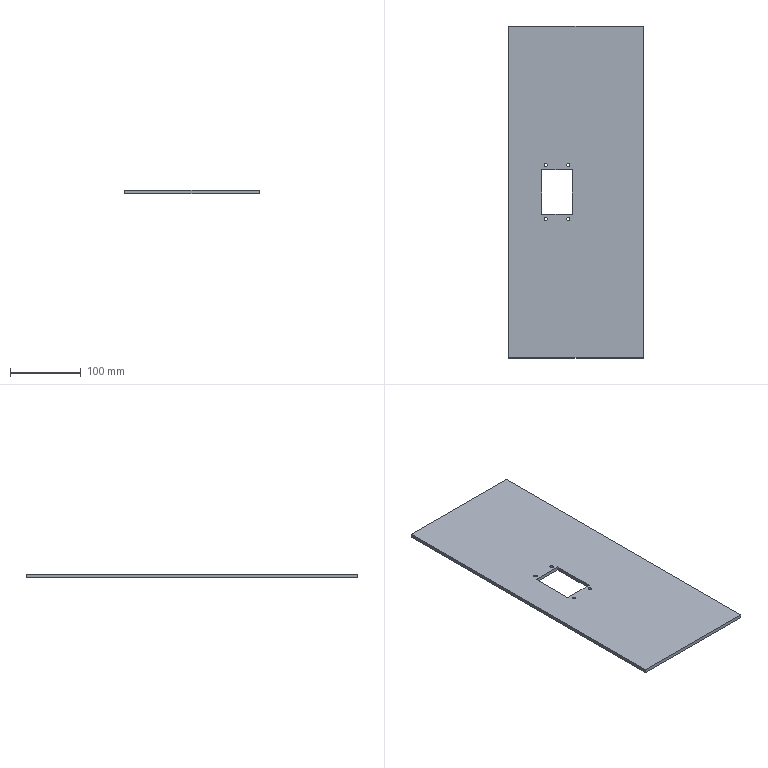Part | NX | features BREP 1 | 1 solid | 18 faces | box 189.5 x 468.1 x 5 mm | volume 429662 mm3 | plane 10 | cylinder 8 | commonest cylinder face diameters 4.5 x8
STEP:
#1=CARTESIAN_POINT('',(-13.,-38.,-2.5));
#2=VERTEX_POINT('',#1);
#3=CARTESIAN_POINT('',(-8.5,-38.,-2.5));
#4=VERTEX_POINT('',#3);
#5=CARTESIAN_POINT('',(-10.75,-38.,-2.5));
#6=DIRECTION('',(0.,0.,1.));
#7=DIRECTION('',(1.,0.,0.));
#8=AXIS2_PLACEMENT_3D('',#5,#6,#7);
#9=CIRCLE('',#8,2.25);
#10=EDGE_CURVE('',#2,#4,#9,.T.);
#11=ORIENTED_EDGE('',*,*,#10,.F.);
#12=CARTESIAN_POINT('',(-13.,-38.,2.5));
#13=VERTEX_POINT('',#12);
#14=CARTESIAN_POINT('',(-13.,-38.,-2.5));
#15=DIRECTION('',(0.,0.,1.));
#16=VECTOR('',#15,1000.);
#17=LINE('',#14,#16);
#18=EDGE_CURVE('',#13,#2,#17,.F.);
#19=ORIENTED_EDGE('',*,*,#18,.F.);
#20=CARTESIAN_POINT('',(-8.5,-38.,2.5));
#21=VERTEX_POINT('',#20);
#22=CARTESIAN_POINT('',(-10.75,-38.,2.5));
#23=DIRECTION('',(0.,0.,1.));
#24=DIRECTION('',(1.,0.,0.));
#25=AXIS2_PLACEMENT_3D('',#22,#23,#24);
#26=CIRCLE('',#25,2.25);
#27=EDGE_CURVE('',#13,#21,#26,.T.);
#28=ORIENTED_EDGE('',*,*,#27,.T.);
#29=CARTESIAN_POINT('',(-8.5,-38.,-2.5));
#30=DIRECTION('',(0.,0.,1.));
#31=VECTOR('',#30,1000.);
#32=LINE('',#29,#31);
#33=EDGE_CURVE('',#21,#4,#32,.F.);
#34=ORIENTED_EDGE('',*,*,#33,.T.);
#35=EDGE_LOOP('',(#11,#19,#28,#34));
#36=FACE_BOUND('',#35,.T.);
#37=CARTESIAN_POINT('',(-10.75,-38.,-2.5));
#38=DIRECTION('',(0.,0.,1.));
#39=DIRECTION('',(1.,0.,0.));
#40=AXIS2_PLACEMENT_3D('',#37,#38,#39);
#41=CYLINDRICAL_SURFACE('',#40,2.25);
#42=ADVANCED_FACE('',(#36),#41,.F.);
#43=CARTESIAN_POINT('',(-45.,-38.,-2.5));
#44=VERTEX_POINT('',#43);
#45=CARTESIAN_POINT('',(-40.5,-38.,-2.5));
#46=VERTEX_POINT('',#45);
#47=CARTESIAN_POINT('',(-42.75,-38.,-2.5));
#48=DIRECTION('',(0.,0.,1.));
#49=DIRECTION('',(1.,0.,0.));
#50=AXIS2_PLACEMENT_3D('',#47,#48,#49);
#51=CIRCLE('',#50,2.25);
#52=EDGE_CURVE('',#44,#46,#51,.T.);
#53=ORIENTED_EDGE('',*,*,#52,.F.);
#54=CARTESIAN_POINT('',(-45.,-38.,2.5));
#55=VERTEX_POINT('',#54);
#56=CARTESIAN_POINT('',(-45.,-38.,-2.5));
#57=DIRECTION('',(0.,0.,1.));
#58=VECTOR('',#57,1000.);
#59=LINE('',#56,#58);
#60=EDGE_CURVE('',#55,#44,#59,.F.);
#61=ORIENTED_EDGE('',*,*,#60,.F.);
#62=CARTESIAN_POINT('',(-40.5,-38.,2.5));
#63=VERTEX_POINT('',#62);
#64=CARTESIAN_POINT('',(-42.75,-38.,2.5));
#65=DIRECTION('',(0.,0.,1.));
#66=DIRECTION('',(1.,0.,0.));
#67=AXIS2_PLACEMENT_3D('',#64,#65,#66);
#68=CIRCLE('',#67,2.25);
#69=EDGE_CURVE('',#55,#63,#68,.T.);
#70=ORIENTED_EDGE('',*,*,#69,.T.);
#71=CARTESIAN_POINT('',(-40.5,-38.,-2.5));
#72=DIRECTION('',(0.,0.,1.));
#73=VECTOR('',#72,1000.);
#74=LINE('',#71,#73);
#75=EDGE_CURVE('',#63,#46,#74,.F.);
#76=ORIENTED_EDGE('',*,*,#75,.T.);
#77=EDGE_LOOP('',(#53,#61,#70,#76));
#78=FACE_BOUND('',#77,.T.);
#79=CARTESIAN_POINT('',(-42.75,-38.,-2.5));
#80=DIRECTION('',(0.,0.,1.));
#81=DIRECTION('',(1.,0.,0.));
#82=AXIS2_PLACEMENT_3D('',#79,#80,#81);
#83=CYLINDRICAL_SURFACE('',#82,2.25);
#84=ADVANCED_FACE('',(#78),#83,.F.);
#85=CARTESIAN_POINT('',(-13.,38.,-2.5));
#86=VERTEX_POINT('',#85);
#87=CARTESIAN_POINT('',(-8.5,38.,-2.5));
#88=VERTEX_POINT('',#87);
#89=CARTESIAN_POINT('',(-10.75,38.,-2.5));
#90=DIRECTION('',(0.,0.,1.));
#91=DIRECTION('',(1.,0.,0.));
#92=AXIS2_PLACEMENT_3D('',#89,#90,#91);
#93=CIRCLE('',#92,2.25);
#94=EDGE_CURVE('',#86,#88,#93,.T.);
#95=ORIENTED_EDGE('',*,*,#94,.F.);
#96=CARTESIAN_POINT('',(-13.,38.,2.5));
#97=VERTEX_POINT('',#96);
#98=CARTESIAN_POINT('',(-13.,38.,-2.5));
#99=DIRECTION('',(0.,0.,1.));
#100=VECTOR('',#99,1000.);
#101=LINE('',#98,#100);
#102=EDGE_CURVE('',#97,#86,#101,.F.);
#103=ORIENTED_EDGE('',*,*,#102,.F.);
#104=CARTESIAN_POINT('',(-8.5,38.,2.5));
#105=VERTEX_POINT('',#104);
#106=CARTESIAN_POINT('',(-10.75,38.,2.5));
#107=DIRECTION('',(0.,0.,1.));
#108=DIRECTION('',(1.,0.,0.));
#109=AXIS2_PLACEMENT_3D('',#106,#107,#108);
#110=CIRCLE('',#109,2.25);
#111=EDGE_CURVE('',#97,#105,#110,.T.);
#112=ORIENTED_EDGE('',*,*,#111,.T.);
#113=CARTESIAN_POINT('',(-8.5,38.,-2.5));
#114=DIRECTION('',(0.,0.,1.));
#115=VECTOR('',#114,1000.);
#116=LINE('',#113,#115);
#117=EDGE_CURVE('',#105,#88,#116,.F.);
#118=ORIENTED_EDGE('',*,*,#117,.T.);
#119=EDGE_LOOP('',(#95,#103,#112,#118));
#120=FACE_BOUND('',#119,.T.);
#121=CARTESIAN_POINT('',(-10.75,38.,-2.5));
#122=DIRECTION('',(0.,0.,1.));
#123=DIRECTION('',(1.,0.,0.));
#124=AXIS2_PLACEMENT_3D('',#121,#122,#123);
#125=CYLINDRICAL_SURFACE('',#124,2.25);
#126=ADVANCED_FACE('',(#120),#125,.F.);
#127=CARTESIAN_POINT('',(-45.,38.,-2.5));
#128=VERTEX_POINT('',#127);
#129=CARTESIAN_POINT('',(-40.5,38.,-2.5));
#130=VERTEX_POINT('',#129);
#131=CARTESIAN_POINT('',(-42.75,38.,-2.5));
#132=DIRECTION('',(0.,0.,1.));
#133=DIRECTION('',(1.,0.,0.));
#134=AXIS2_PLACEMENT_3D('',#131,#132,#133);
#135=CIRCLE('',#134,2.25);
#136=EDGE_CURVE('',#128,#130,#135,.T.);
#137=ORIENTED_EDGE('',*,*,#136,.F.);
#138=CARTESIAN_POINT('',(-45.,38.,2.5));
#139=VERTEX_POINT('',#138);
#140=CARTESIAN_POINT('',(-45.,38.,-2.5));
#141=DIRECTION('',(0.,0.,1.));
#142=VECTOR('',#141,1000.);
#143=LINE('',#140,#142);
#144=EDGE_CURVE('',#139,#128,#143,.F.);
#145=ORIENTED_EDGE('',*,*,#144,.F.);
#146=CARTESIAN_POINT('',(-40.5,38.,2.5));
#147=VERTEX_POINT('',#146);
#148=CARTESIAN_POINT('',(-42.75,38.,2.5));
#149=DIRECTION('',(0.,0.,1.));
#150=DIRECTION('',(1.,0.,0.));
#151=AXIS2_PLACEMENT_3D('',#148,#149,#150);
#152=CIRCLE('',#151,2.25);
#153=EDGE_CURVE('',#139,#147,#152,.T.);
#154=ORIENTED_EDGE('',*,*,#153,.T.);
#155=CARTESIAN_POINT('',(-40.5,38.,-2.5));
#156=DIRECTION('',(0.,0.,1.));
#157=VECTOR('',#156,1000.);
#158=LINE('',#155,#157);
#159=EDGE_CURVE('',#147,#130,#158,.F.);
#160=ORIENTED_EDGE('',*,*,#159,.T.);
#161=EDGE_LOOP('',(#137,#145,#154,#160));
#162=FACE_BOUND('',#161,.T.);
#163=CARTESIAN_POINT('',(-42.75,38.,-2.5));
#164=DIRECTION('',(0.,0.,1.));
#165=DIRECTION('',(1.,0.,0.));
#166=AXIS2_PLACEMENT_3D('',#163,#164,#165);
#167=CYLINDRICAL_SURFACE('',#166,2.25);
#168=ADVANCED_FACE('',(#162),#167,.F.);
#169=CARTESIAN_POINT('',(94.75,-234.05,-2.5));
#170=VERTEX_POINT('',#169);
#171=CARTESIAN_POINT('',(94.75,234.05,-2.5));
#172=VERTEX_POINT('',#171);
#173=CARTESIAN_POINT('',(94.75,-234.05,-2.5));
#174=DIRECTION('',(0.,1.,0.));
#175=VECTOR('',#174,1000.);
#176=LINE('',#173,#175);
#177=EDGE_CURVE('',#170,#172,#176,.T.);
#178=ORIENTED_EDGE('',*,*,#177,.T.);
#179=CARTESIAN_POINT('',(94.75,234.05,2.5));
#180=VERTEX_POINT('',#179);
#181=CARTESIAN_POINT('',(94.75,234.05,2.5));
#182=DIRECTION('',(0.,0.,-1.));
#183=VECTOR('',#182,1000.);
#184=LINE('',#181,#183);
#185=EDGE_CURVE('',#180,#172,#184,.T.);
#186=ORIENTED_EDGE('',*,*,#185,.F.);
#187=CARTESIAN_POINT('',(94.75,-234.05,2.5));
#188=VERTEX_POINT('',#187);
#189=CARTESIAN_POINT('',(94.75,-234.05,2.5));
#190=DIRECTION('',(0.,1.,0.));
#191=VECTOR('',#190,1000.);
#192=LINE('',#189,#191);
#193=EDGE_CURVE('',#188,#180,#192,.T.);
#194=ORIENTED_EDGE('',*,*,#193,.F.);
#195=CARTESIAN_POINT('',(94.75,-234.05,2.5));
#196=DIRECTION('',(0.,0.,-1.));
#197=VECTOR('',#196,1000.);
#198=LINE('',#195,#197);
#199=EDGE_CURVE('',#188,#170,#198,.T.);
#200=ORIENTED_EDGE('',*,*,#199,.T.);
#201=EDGE_LOOP('',(#178,#186,#194,#200));
#202=FACE_BOUND('',#201,.T.);
#203=CARTESIAN_POINT('',(94.75,-234.05,2.5));
#204=DIRECTION('',(-1.,0.,0.));
#205=DIRECTION('',(0.,0.,1.));
#206=AXIS2_PLACEMENT_3D('',#203,#204,#205);
#207=PLANE('',#206);
#208=ADVANCED_FACE('',(#202),#207,.F.);
#209=CARTESIAN_POINT('',(-94.75,234.05,-2.5));
#210=VERTEX_POINT('',#209);
#211=CARTESIAN_POINT('',(-94.75,234.05,-2.5));
#212=DIRECTION('',(-1.,0.,0.));
#213=VECTOR('',#212,1000.);
#214=LINE('',#211,#213);
#215=EDGE_CURVE('',#172,#210,#214,.T.);
#216=ORIENTED_EDGE('',*,*,#215,.T.);
#217=CARTESIAN_POINT('',(-94.75,234.05,2.5));
#218=VERTEX_POINT('',#217);
#219=CARTESIAN_POINT('',(-94.75,234.05,2.5));
#220=DIRECTION('',(0.,0.,-1.));
#221=VECTOR('',#220,1000.);
#222=LINE('',#219,#221);
#223=EDGE_CURVE('',#218,#210,#222,.T.);
#224=ORIENTED_EDGE('',*,*,#223,.F.);
#225=CARTESIAN_POINT('',(-94.75,234.05,2.5));
#226=DIRECTION('',(-1.,0.,0.));
#227=VECTOR('',#226,1000.);
#228=LINE('',#225,#227);
#229=EDGE_CURVE('',#180,#218,#228,.T.);
#230=ORIENTED_EDGE('',*,*,#229,.F.);
#231=ORIENTED_EDGE('',*,*,#185,.T.);
#232=EDGE_LOOP('',(#216,#224,#230,#231));
#233=FACE_BOUND('',#232,.T.);
#234=CARTESIAN_POINT('',(-94.75,234.05,2.5));
#235=DIRECTION('',(0.,-1.,0.));
#236=DIRECTION('',(0.,0.,-1.));
#237=AXIS2_PLACEMENT_3D('',#234,#235,#236);
#238=PLANE('',#237);
#239=ADVANCED_FACE('',(#233),#238,.F.);
#240=CARTESIAN_POINT('',(-94.75,-234.05,-2.5));
#241=VERTEX_POINT('',#240);
#242=CARTESIAN_POINT('',(-94.75,-234.05,-2.5));
#243=DIRECTION('',(0.,-1.,0.));
#244=VECTOR('',#243,1000.);
#245=LINE('',#242,#244);
#246=EDGE_CURVE('',#210,#241,#245,.T.);
#247=ORIENTED_EDGE('',*,*,#246,.T.);
#248=CARTESIAN_POINT('',(-94.75,-234.05,2.5));
#249=VERTEX_POINT('',#248);
#250=CARTESIAN_POINT('',(-94.75,-234.05,2.5));
#251=DIRECTION('',(0.,0.,-1.));
#252=VECTOR('',#251,1000.);
#253=LINE('',#250,#252);
#254=EDGE_CURVE('',#249,#241,#253,.T.);
#255=ORIENTED_EDGE('',*,*,#254,.F.);
#256=CARTESIAN_POINT('',(-94.75,-234.05,2.5));
#257=DIRECTION('',(0.,-1.,0.));
#258=VECTOR('',#257,1000.);
#259=LINE('',#256,#258);
#260=EDGE_CURVE('',#218,#249,#259,.T.);
#261=ORIENTED_EDGE('',*,*,#260,.F.);
#262=ORIENTED_EDGE('',*,*,#223,.T.);
#263=EDGE_LOOP('',(#247,#255,#261,#262));
#264=FACE_BOUND('',#263,.T.);
#265=CARTESIAN_POINT('',(-94.75,-234.05,2.5));
#266=DIRECTION('',(1.,0.,0.));
#267=DIRECTION('',(0.,1.,0.));
#268=AXIS2_PLACEMENT_3D('',#265,#266,#267);
#269=PLANE('',#268);
#270=ADVANCED_FACE('',(#264),#269,.F.);
#271=CARTESIAN_POINT('',(-94.75,-234.05,-2.5));
#272=DIRECTION('',(1.,0.,0.));
#273=VECTOR('',#272,1000.);
#274=LINE('',#271,#273);
#275=EDGE_CURVE('',#241,#170,#274,.T.);
#276=ORIENTED_EDGE('',*,*,#275,.T.);
#277=ORIENTED_EDGE('',*,*,#199,.F.);
#278=CARTESIAN_POINT('',(-94.75,-234.05,2.5));
#279=DIRECTION('',(1.,0.,0.));
#280=VECTOR('',#279,1000.);
#281=LINE('',#278,#280);
#282=EDGE_CURVE('',#249,#188,#281,.T.);
#283=ORIENTED_EDGE('',*,*,#282,.F.);
#284=ORIENTED_EDGE('',*,*,#254,.T.);
#285=EDGE_LOOP('',(#276,#277,#283,#284));
#286=FACE_BOUND('',#285,.T.);
#287=CARTESIAN_POINT('',(-94.75,-234.05,2.5));
#288=DIRECTION('',(0.,1.,0.));
#289=DIRECTION('',(1.,0.,0.));
#290=AXIS2_PLACEMENT_3D('',#287,#288,#289);
#291=PLANE('',#290);
#292=ADVANCED_FACE('',(#286),#291,.F.);
#293=ORIENTED_EDGE('',*,*,#193,.T.);
#294=ORIENTED_EDGE('',*,*,#229,.T.);
#295=ORIENTED_EDGE('',*,*,#260,.T.);
#296=ORIENTED_EDGE('',*,*,#282,.T.);
#297=EDGE_LOOP('',(#293,#294,#295,#296));
#298=FACE_BOUND('',#297,.T.);
#299=CARTESIAN_POINT('',(-10.75,-38.,2.5));
#300=DIRECTION('',(0.,0.,1.));
#301=DIRECTION('',(1.,0.,0.));
#302=AXIS2_PLACEMENT_3D('',#299,#300,#301);
#303=CIRCLE('',#302,2.25);
#304=EDGE_CURVE('',#21,#13,#303,.T.);
#305=ORIENTED_EDGE('',*,*,#304,.F.);
#306=ORIENTED_EDGE('',*,*,#27,.F.);
#307=EDGE_LOOP('',(#305,#306));
#308=FACE_BOUND('',#307,.T.);
#309=CARTESIAN_POINT('',(-42.75,-38.,2.5));
#310=DIRECTION('',(0.,0.,1.));
#311=DIRECTION('',(1.,0.,0.));
#312=AXIS2_PLACEMENT_3D('',#309,#310,#311);
#313=CIRCLE('',#312,2.25);
#314=EDGE_CURVE('',#63,#55,#313,.T.);
#315=ORIENTED_EDGE('',*,*,#314,.F.);
#316=ORIENTED_EDGE('',*,*,#69,.F.);
#317=EDGE_LOOP('',(#315,#316));
#318=FACE_BOUND('',#317,.T.);
#319=CARTESIAN_POINT('',(-10.75,38.,2.5));
#320=DIRECTION('',(0.,0.,1.));
#321=DIRECTION('',(1.,0.,0.));
#322=AXIS2_PLACEMENT_3D('',#319,#320,#321);
#323=CIRCLE('',#322,2.25);
#324=EDGE_CURVE('',#105,#97,#323,.T.);
#325=ORIENTED_EDGE('',*,*,#324,.F.);
#326=ORIENTED_EDGE('',*,*,#111,.F.);
#327=EDGE_LOOP('',(#325,#326));
#328=FACE_BOUND('',#327,.T.);
#329=CARTESIAN_POINT('',(-42.75,38.,2.5));
#330=DIRECTION('',(0.,0.,1.));
#331=DIRECTION('',(1.,0.,0.));
#332=AXIS2_PLACEMENT_3D('',#329,#330,#331);
#333=CIRCLE('',#332,2.25);
#334=EDGE_CURVE('',#147,#139,#333,.T.);
#335=ORIENTED_EDGE('',*,*,#334,.F.);
#336=ORIENTED_EDGE('',*,*,#153,.F.);
#337=EDGE_LOOP('',(#335,#336));
#338=FACE_BOUND('',#337,.T.);
#339=CARTESIAN_POINT('',(-5.25,31.5,2.5));
#340=VERTEX_POINT('',#339);
#341=CARTESIAN_POINT('',(-48.25,31.5,2.5));
#342=VERTEX_POINT('',#341);
#343=CARTESIAN_POINT('',(-48.25,31.5,2.5));
#344=DIRECTION('',(-1.,0.,0.));
#345=VECTOR('',#344,1000.);
#346=LINE('',#343,#345);
#347=EDGE_CURVE('',#340,#342,#346,.T.);
#348=ORIENTED_EDGE('',*,*,#347,.F.);
#349=CARTESIAN_POINT('',(-5.25,-31.5,2.5));
#350=VERTEX_POINT('',#349);
#351=CARTESIAN_POINT('',(-5.25,-31.5,2.5));
#352=DIRECTION('',(0.,1.,0.));
#353=VECTOR('',#352,1000.);
#354=LINE('',#351,#353);
#355=EDGE_CURVE('',#350,#340,#354,.T.);
#356=ORIENTED_EDGE('',*,*,#355,.F.);
#357=CARTESIAN_POINT('',(-48.25,-31.5,2.5));
#358=VERTEX_POINT('',#357);
#359=CARTESIAN_POINT('',(-48.25,-31.5,2.5));
#360=DIRECTION('',(1.,0.,0.));
#361=VECTOR('',#360,1000.);
#362=LINE('',#359,#361);
#363=EDGE_CURVE('',#358,#350,#362,.T.);
#364=ORIENTED_EDGE('',*,*,#363,.F.);
#365=CARTESIAN_POINT('',(-48.25,-31.5,2.5));
#366=DIRECTION('',(0.,-1.,0.));
#367=VECTOR('',#366,1000.);
#368=LINE('',#365,#367);
#369=EDGE_CURVE('',#342,#358,#368,.T.);
#370=ORIENTED_EDGE('',*,*,#369,.F.);
#371=EDGE_LOOP('',(#348,#356,#364,#370));
#372=FACE_BOUND('',#371,.T.);
#373=CARTESIAN_POINT('',(0.,0.,2.5));
#374=DIRECTION('',(0.,0.,-1.));
#375=DIRECTION('',(0.,-1.,0.));
#376=AXIS2_PLACEMENT_3D('',#373,#374,#375);
#377=PLANE('',#376);
#378=ADVANCED_FACE('',(#298,#308,#318,#328,#338,#372),#377,.F.);
#379=ORIENTED_EDGE('',*,*,#177,.F.);
#380=ORIENTED_EDGE('',*,*,#275,.F.);
#381=ORIENTED_EDGE('',*,*,#246,.F.);
#382=ORIENTED_EDGE('',*,*,#215,.F.);
#383=EDGE_LOOP('',(#379,#380,#381,#382));
#384=FACE_BOUND('',#383,.T.);
#385=CARTESIAN_POINT('',(-10.75,-38.,-2.5));
#386=DIRECTION('',(0.,0.,1.));
#387=DIRECTION('',(1.,0.,0.));
#388=AXIS2_PLACEMENT_3D('',#385,#386,#387);
#389=CIRCLE('',#388,2.25);
#390=EDGE_CURVE('',#4,#2,#389,.T.);
#391=ORIENTED_EDGE('',*,*,#390,.T.);
#392=ORIENTED_EDGE('',*,*,#10,.T.);
#393=EDGE_LOOP('',(#391,#392));
#394=FACE_BOUND('',#393,.T.);
#395=CARTESIAN_POINT('',(-42.75,-38.,-2.5));
#396=DIRECTION('',(0.,0.,1.));
#397=DIRECTION('',(1.,0.,0.));
#398=AXIS2_PLACEMENT_3D('',#395,#396,#397);
#399=CIRCLE('',#398,2.25);
#400=EDGE_CURVE('',#46,#44,#399,.T.);
#401=ORIENTED_EDGE('',*,*,#400,.T.);
#402=ORIENTED_EDGE('',*,*,#52,.T.);
#403=EDGE_LOOP('',(#401,#402));
#404=FACE_BOUND('',#403,.T.);
#405=CARTESIAN_POINT('',(-10.75,38.,-2.5));
#406=DIRECTION('',(0.,0.,1.));
#407=DIRECTION('',(1.,0.,0.));
#408=AXIS2_PLACEMENT_3D('',#405,#406,#407);
#409=CIRCLE('',#408,2.25);
#410=EDGE_CURVE('',#88,#86,#409,.T.);
#411=ORIENTED_EDGE('',*,*,#410,.T.);
#412=ORIENTED_EDGE('',*,*,#94,.T.);
#413=EDGE_LOOP('',(#411,#412));
#414=FACE_BOUND('',#413,.T.);
#415=CARTESIAN_POINT('',(-42.75,38.,-2.5));
#416=DIRECTION('',(0.,0.,1.));
#417=DIRECTION('',(1.,0.,0.));
#418=AXIS2_PLACEMENT_3D('',#415,#416,#417);
#419=CIRCLE('',#418,2.25);
#420=EDGE_CURVE('',#130,#128,#419,.T.);
#421=ORIENTED_EDGE('',*,*,#420,.T.);
#422=ORIENTED_EDGE('',*,*,#136,.T.);
#423=EDGE_LOOP('',(#421,#422));
#424=FACE_BOUND('',#423,.T.);
#425=CARTESIAN_POINT('',(-5.25,-31.5,-2.5));
#426=VERTEX_POINT('',#425);
#427=CARTESIAN_POINT('',(-5.25,31.5,-2.5));
#428=VERTEX_POINT('',#427);
#429=CARTESIAN_POINT('',(-5.25,-31.5,-2.5));
#430=DIRECTION('',(0.,1.,0.));
#431=VECTOR('',#430,1000.);
#432=LINE('',#429,#431);
#433=EDGE_CURVE('',#426,#428,#432,.T.);
#434=ORIENTED_EDGE('',*,*,#433,.T.);
#435=CARTESIAN_POINT('',(-48.25,31.5,-2.5));
#436=VERTEX_POINT('',#435);
#437=CARTESIAN_POINT('',(-48.25,31.5,-2.5));
#438=DIRECTION('',(-1.,0.,0.));
#439=VECTOR('',#438,1000.);
#440=LINE('',#437,#439);
#441=EDGE_CURVE('',#428,#436,#440,.T.);
#442=ORIENTED_EDGE('',*,*,#441,.T.);
#443=CARTESIAN_POINT('',(-48.25,-31.5,-2.5));
#444=VERTEX_POINT('',#443);
#445=CARTESIAN_POINT('',(-48.25,-31.5,-2.5));
#446=DIRECTION('',(0.,-1.,0.));
#447=VECTOR('',#446,1000.);
#448=LINE('',#445,#447);
#449=EDGE_CURVE('',#436,#444,#448,.T.);
#450=ORIENTED_EDGE('',*,*,#449,.T.);
#451=CARTESIAN_POINT('',(-48.25,-31.5,-2.5));
#452=DIRECTION('',(1.,0.,0.));
#453=VECTOR('',#452,1000.);
#454=LINE('',#451,#453);
#455=EDGE_CURVE('',#444,#426,#454,.T.);
#456=ORIENTED_EDGE('',*,*,#455,.T.);
#457=EDGE_LOOP('',(#434,#442,#450,#456));
#458=FACE_BOUND('',#457,.T.);
#459=CARTESIAN_POINT('',(0.,0.,-2.5));
#460=DIRECTION('',(0.,0.,-1.));
#461=DIRECTION('',(0.,-1.,0.));
#462=AXIS2_PLACEMENT_3D('',#459,#460,#461);
#463=PLANE('',#462);
#464=ADVANCED_FACE('',(#384,#394,#404,#414,#424,#458),#463,.T.);
#465=CARTESIAN_POINT('',(-5.25,31.5,-2.5));
#466=DIRECTION('',(0.,0.,1.));
#467=VECTOR('',#466,1000.);
#468=LINE('',#465,#467);
#469=EDGE_CURVE('',#428,#340,#468,.T.);
#470=ORIENTED_EDGE('',*,*,#469,.F.);
#471=ORIENTED_EDGE('',*,*,#433,.F.);
#472=CARTESIAN_POINT('',(-5.25,-31.5,-2.5));
#473=DIRECTION('',(0.,0.,1.));
#474=VECTOR('',#473,1000.);
#475=LINE('',#472,#474);
#476=EDGE_CURVE('',#426,#350,#475,.T.);
#477=ORIENTED_EDGE('',*,*,#476,.T.);
#478=ORIENTED_EDGE('',*,*,#355,.T.);
#479=EDGE_LOOP('',(#470,#471,#477,#478));
#480=FACE_BOUND('',#479,.T.);
#481=CARTESIAN_POINT('',(-5.25,-31.5,-2.5));
#482=DIRECTION('',(1.,0.,0.));
#483=DIRECTION('',(0.,1.,0.));
#484=AXIS2_PLACEMENT_3D('',#481,#482,#483);
#485=PLANE('',#484);
#486=ADVANCED_FACE('',(#480),#485,.F.);
#487=ORIENTED_EDGE('',*,*,#476,.F.);
#488=ORIENTED_EDGE('',*,*,#455,.F.);
#489=CARTESIAN_POINT('',(-48.25,-31.5,-2.5));
#490=DIRECTION('',(0.,0.,1.));
#491=VECTOR('',#490,1000.);
#492=LINE('',#489,#491);
#493=EDGE_CURVE('',#444,#358,#492,.T.);
#494=ORIENTED_EDGE('',*,*,#493,.T.);
#495=ORIENTED_EDGE('',*,*,#363,.T.);
#496=EDGE_LOOP('',(#487,#488,#494,#495));
#497=FACE_BOUND('',#496,.T.);
#498=CARTESIAN_POINT('',(-48.25,-31.5,-2.5));
#499=DIRECTION('',(0.,-1.,0.));
#500=DIRECTION('',(0.,0.,-1.));
#501=AXIS2_PLACEMENT_3D('',#498,#499,#500);
#502=PLANE('',#501);
#503=ADVANCED_FACE('',(#497),#502,.F.);
#504=ORIENTED_EDGE('',*,*,#493,.F.);
#505=ORIENTED_EDGE('',*,*,#449,.F.);
#506=CARTESIAN_POINT('',(-48.25,31.5,-2.5));
#507=DIRECTION('',(0.,0.,1.));
#508=VECTOR('',#507,1000.);
#509=LINE('',#506,#508);
#510=EDGE_CURVE('',#436,#342,#509,.T.);
#511=ORIENTED_EDGE('',*,*,#510,.T.);
#512=ORIENTED_EDGE('',*,*,#369,.T.);
#513=EDGE_LOOP('',(#504,#505,#511,#512));
#514=FACE_BOUND('',#513,.T.);
#515=CARTESIAN_POINT('',(-48.25,-31.5,-2.5));
#516=DIRECTION('',(-1.,0.,0.));
#517=DIRECTION('',(0.,0.,1.));
#518=AXIS2_PLACEMENT_3D('',#515,#516,#517);
#519=PLANE('',#518);
#520=ADVANCED_FACE('',(#514),#519,.F.);
#521=ORIENTED_EDGE('',*,*,#510,.F.);
#522=ORIENTED_EDGE('',*,*,#441,.F.);
#523=ORIENTED_EDGE('',*,*,#469,.T.);
#524=ORIENTED_EDGE('',*,*,#347,.T.);
#525=EDGE_LOOP('',(#521,#522,#523,#524));
#526=FACE_BOUND('',#525,.T.);
#527=CARTESIAN_POINT('',(-48.25,31.5,-2.5));
#528=DIRECTION('',(0.,1.,0.));
#529=DIRECTION('',(1.,0.,0.));
#530=AXIS2_PLACEMENT_3D('',#527,#528,#529);
#531=PLANE('',#530);
#532=ADVANCED_FACE('',(#526),#531,.F.);
#533=ORIENTED_EDGE('',*,*,#144,.T.);
#534=ORIENTED_EDGE('',*,*,#420,.F.);
#535=ORIENTED_EDGE('',*,*,#159,.F.);
#536=ORIENTED_EDGE('',*,*,#334,.T.);
#537=EDGE_LOOP('',(#533,#534,#535,#536));
#538=FACE_BOUND('',#537,.T.);
#539=CARTESIAN_POINT('',(-42.75,38.,-2.5));
#540=DIRECTION('',(0.,0.,1.));
#541=DIRECTION('',(1.,0.,0.));
#542=AXIS2_PLACEMENT_3D('',#539,#540,#541);
#543=CYLINDRICAL_SURFACE('',#542,2.25);
#544=ADVANCED_FACE('',(#538),#543,.F.);
#545=ORIENTED_EDGE('',*,*,#102,.T.);
#546=ORIENTED_EDGE('',*,*,#410,.F.);
#547=ORIENTED_EDGE('',*,*,#117,.F.);
#548=ORIENTED_EDGE('',*,*,#324,.T.);
#549=EDGE_LOOP('',(#545,#546,#547,#548));
#550=FACE_BOUND('',#549,.T.);
#551=CARTESIAN_POINT('',(-10.75,38.,-2.5));
#552=DIRECTION('',(0.,0.,1.));
#553=DIRECTION('',(1.,0.,0.));
#554=AXIS2_PLACEMENT_3D('',#551,#552,#553);
#555=CYLINDRICAL_SURFACE('',#554,2.25);
#556=ADVANCED_FACE('',(#550),#555,.F.);
#557=ORIENTED_EDGE('',*,*,#60,.T.);
#558=ORIENTED_EDGE('',*,*,#400,.F.);
#559=ORIENTED_EDGE('',*,*,#75,.F.);
#560=ORIENTED_EDGE('',*,*,#314,.T.);
#561=EDGE_LOOP('',(#557,#558,#559,#560));
#562=FACE_BOUND('',#561,.T.);
#563=CARTESIAN_POINT('',(-42.75,-38.,-2.5));
#564=DIRECTION('',(0.,0.,1.));
#565=DIRECTION('',(1.,0.,0.));
#566=AXIS2_PLACEMENT_3D('',#563,#564,#565);
#567=CYLINDRICAL_SURFACE('',#566,2.25);
#568=ADVANCED_FACE('',(#562),#567,.F.);
#569=ORIENTED_EDGE('',*,*,#18,.T.);
#570=ORIENTED_EDGE('',*,*,#390,.F.);
#571=ORIENTED_EDGE('',*,*,#33,.F.);
#572=ORIENTED_EDGE('',*,*,#304,.T.);
#573=EDGE_LOOP('',(#569,#570,#571,#572));
#574=FACE_BOUND('',#573,.T.);
#575=CARTESIAN_POINT('',(-10.75,-38.,-2.5));
#576=DIRECTION('',(0.,0.,1.));
#577=DIRECTION('',(1.,0.,0.));
#578=AXIS2_PLACEMENT_3D('',#575,#576,#577);
#579=CYLINDRICAL_SURFACE('',#578,2.25);
#580=ADVANCED_FACE('',(#574),#579,.F.);
#581=CLOSED_SHELL('',(#42,#84,#126,#168,#208,#239,#270,#292,#378,#464,#486,#503,#520,#532,#544,#556,#568,#580));
#582=MANIFOLD_SOLID_BREP('',#581);
#583=(LENGTH_UNIT()NAMED_UNIT(*)SI_UNIT(.MILLI.,.METRE.));
#584=UNCERTAINTY_MEASURE_WITH_UNIT(LENGTH_MEASURE(0.00001),#583,'','');
#585=(NAMED_UNIT(*)PLANE_ANGLE_UNIT()SI_UNIT($,.RADIAN.));
#586=(NAMED_UNIT(*)SI_UNIT($,.STERADIAN.)SOLID_ANGLE_UNIT());
#587=(GEOMETRIC_REPRESENTATION_CONTEXT(3)GLOBAL_UNCERTAINTY_ASSIGNED_CONTEXT((#584))GLOBAL_UNIT_ASSIGNED_CONTEXT((#583,#585,#586))REPRESENTATION_CONTEXT('',''));
#588=ADVANCED_BREP_SHAPE_REPRESENTATION('',(#582),#587);